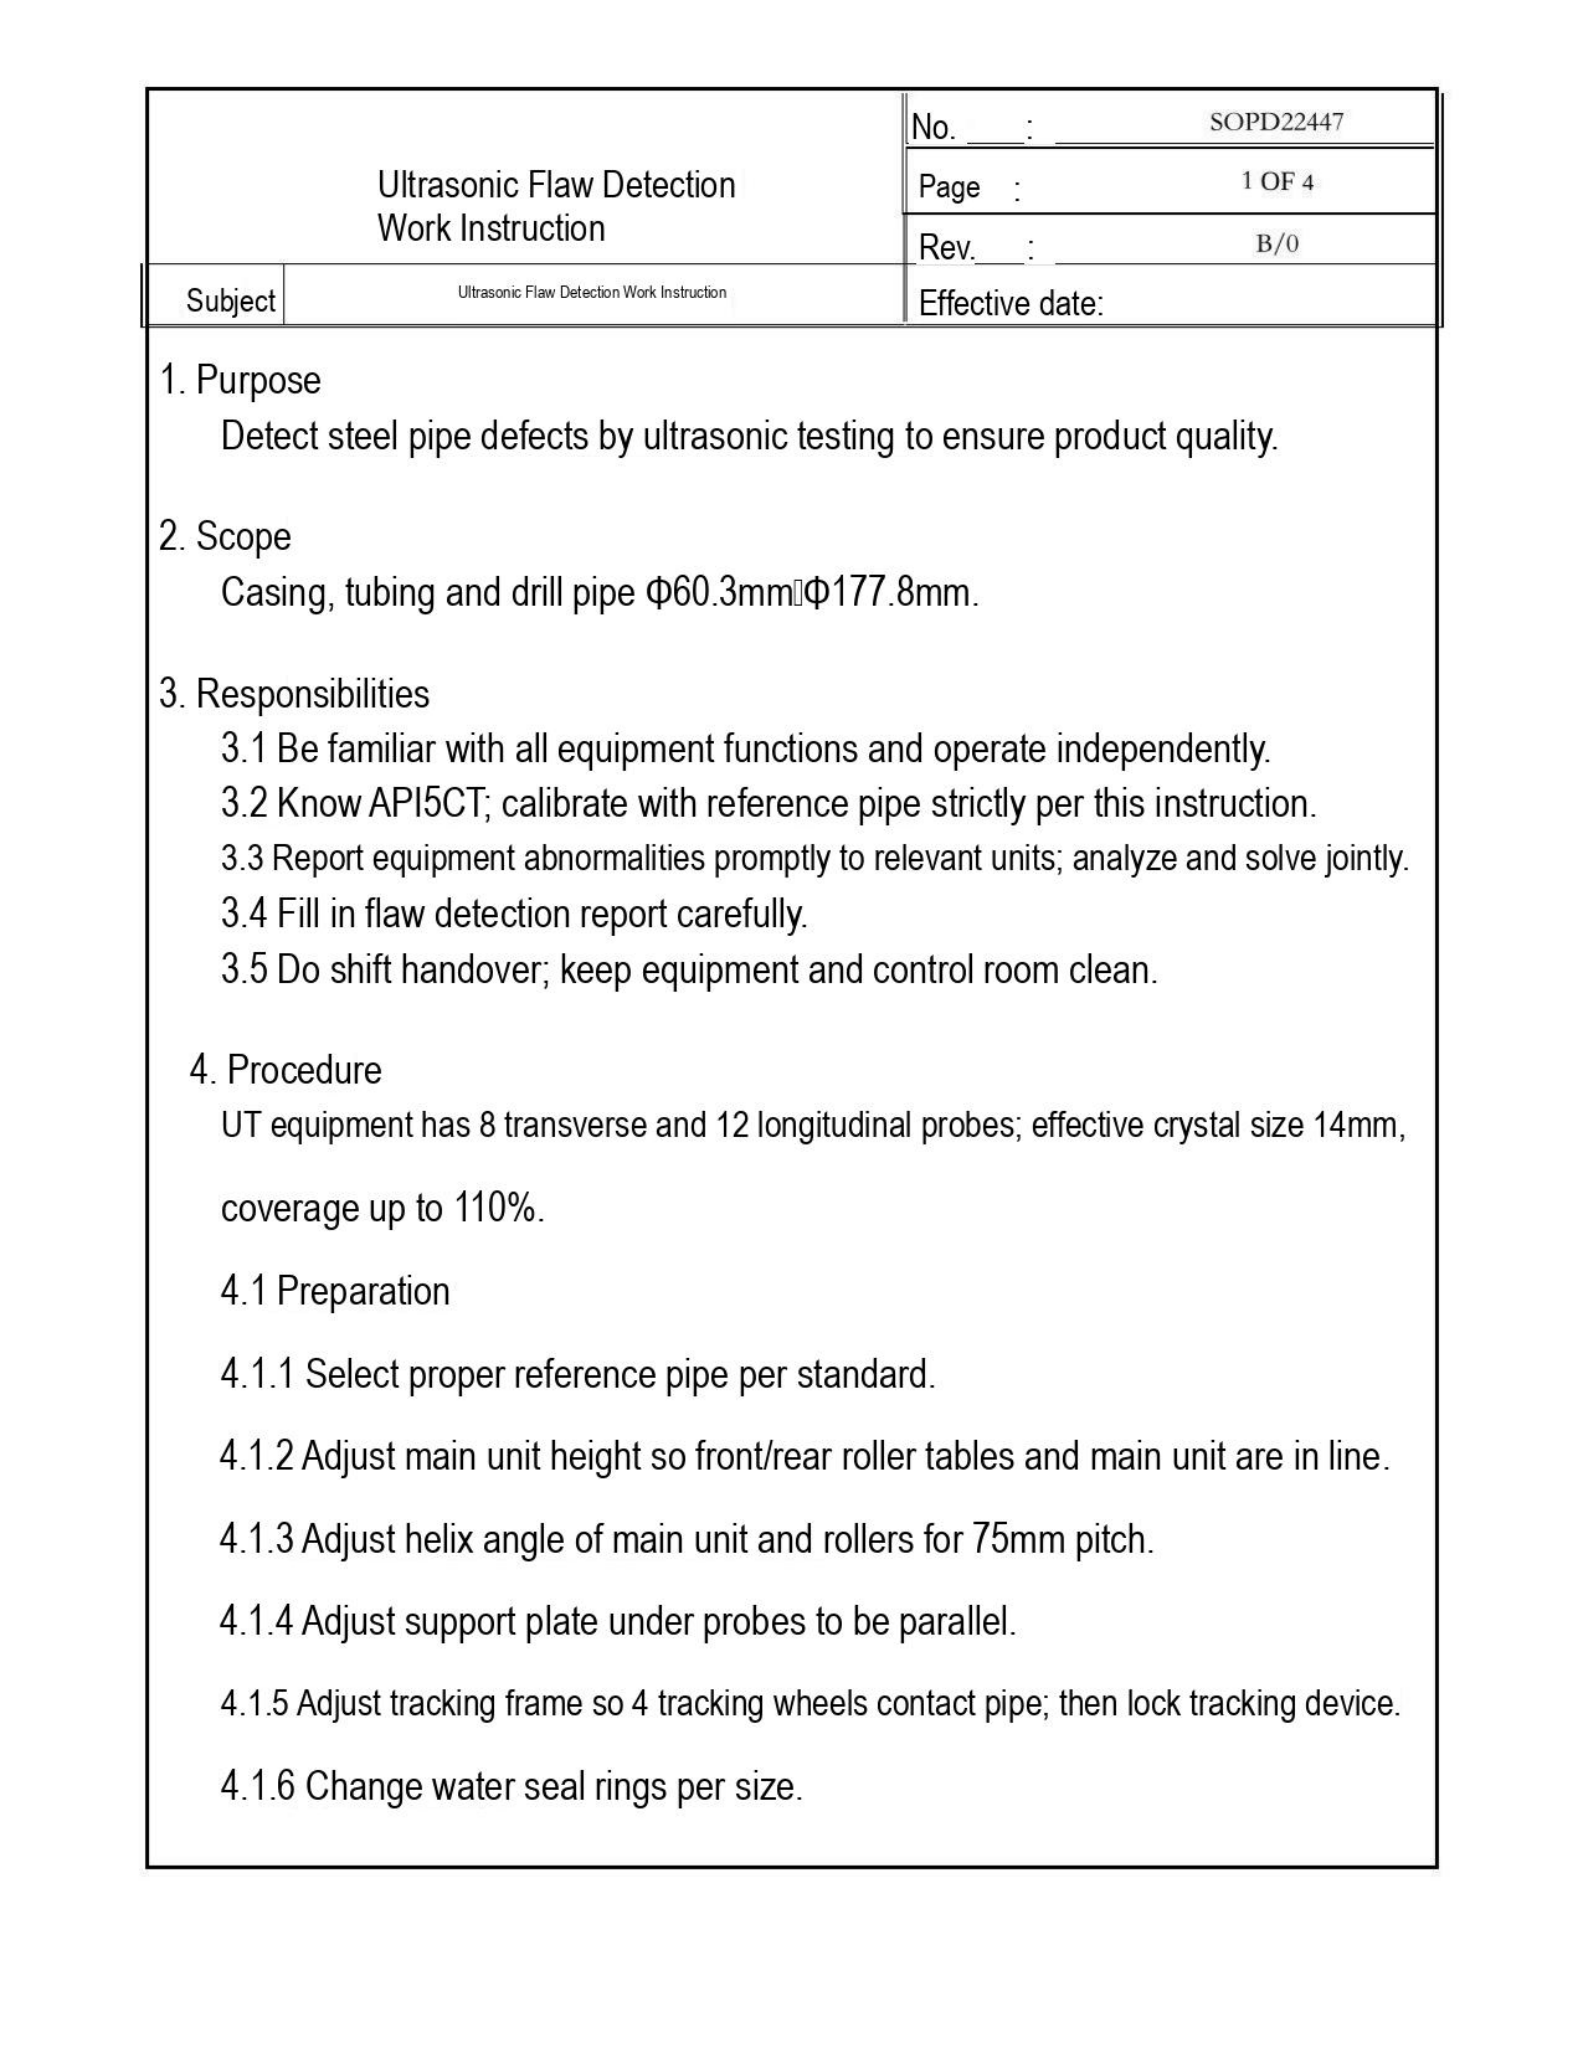| Ultrasonic Flaw Detection Work Instruction | | No. : SOPD22447 |
|---|---|---|
| | | Page : 1 OF 4 |
| | | Rev. : B/0 |
| Subject | Ultrasonic Flaw Detection Work Instruction | Effective date: |

1. Purpose

Detect steel pipe defects by ultrasonic testing to ensure product quality.

2. Scope

Casing, tubing and drill pipe Φ60.3mmΦ177.8mm.

3. Responsibilities

3.1 Be familiar with all equipment functions and operate independently.

3.2 Know API5CT; calibrate with reference pipe strictly per this instruction.

3.3 Report equipment abnormalities promptly to relevant units; analyze and solve jointly.

3.4 Fill in flaw detection report carefully.

3.5 Do shift handover; keep equipment and control room clean.

4. Procedure

UT equipment has 8 transverse and 12 longitudinal probes; effective crystal size 14mm, coverage up to 110%.

4.1 Preparation

4.1.1 Select proper reference pipe per standard.

4.1.2 Adjust main unit height so front/rear roller tables and main unit are in line.

4.1.3 Adjust helix angle of main unit and rollers for 75mm pitch.

4.1.4 Adjust support plate under probes to be parallel.

4.1.5 Adjust tracking frame so 4 tracking wheels contact pipe; then lock tracking device.

4.1.6 Change water seal rings per size.
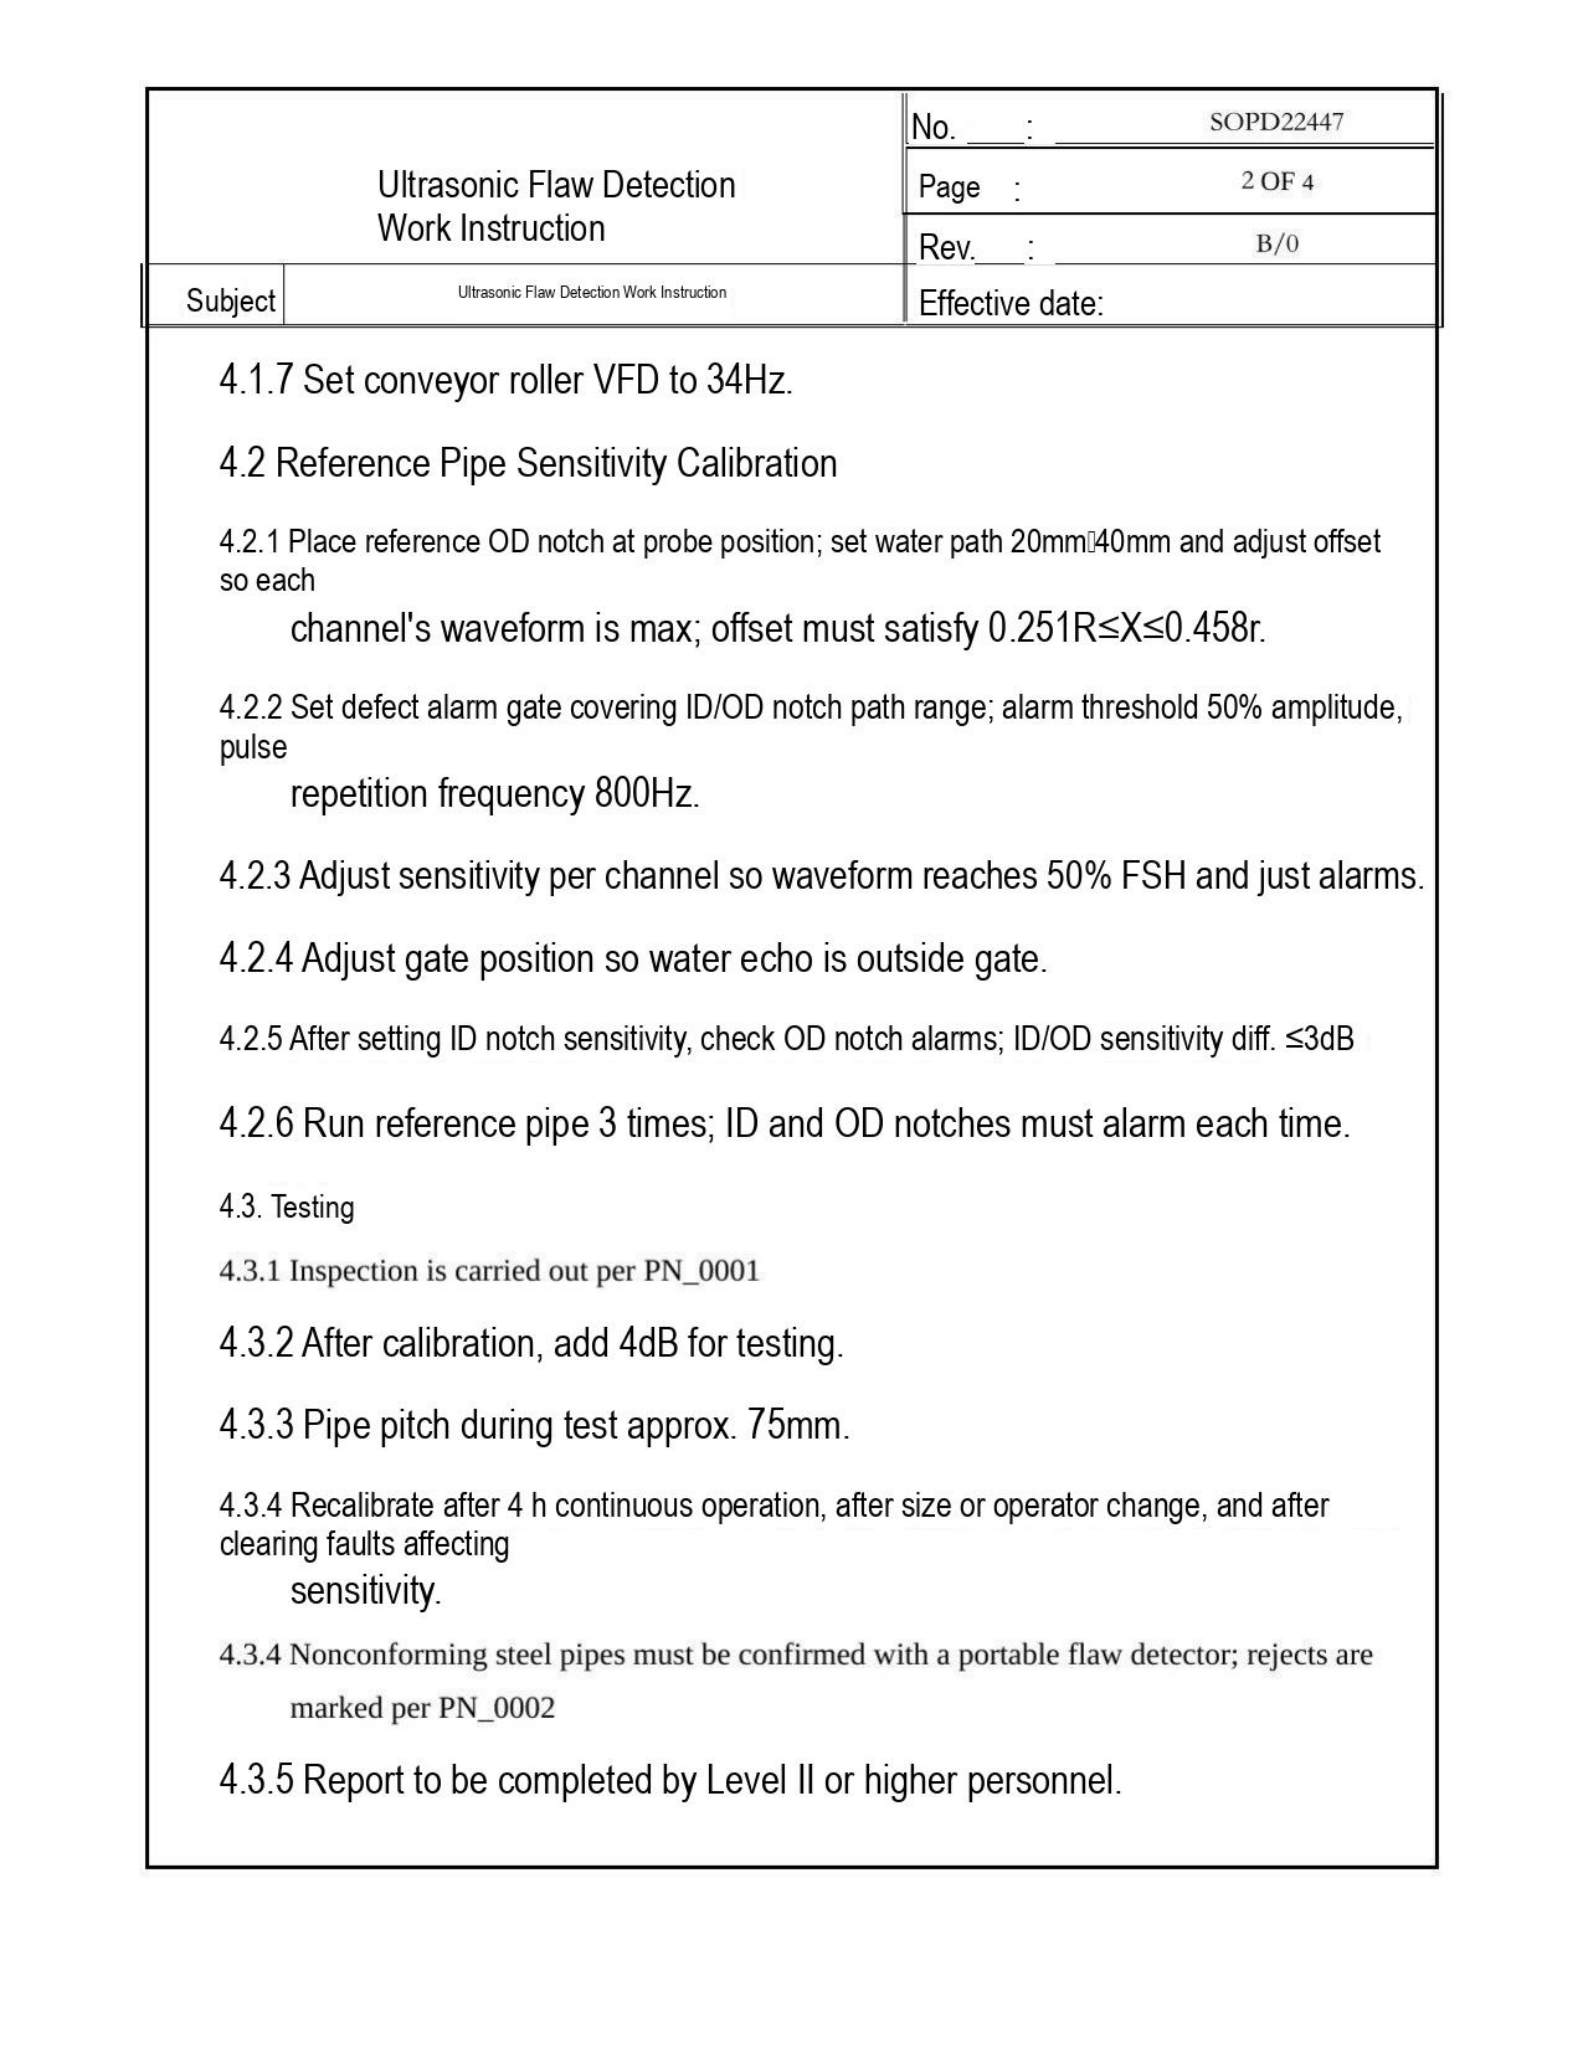| Ultrasonic Flaw Detection Work Instruction | No. : SOPD22447 |
|---|---|
| | Page : 2 OF 4 |
| | Rev. : B/0 |
| Subject: Ultrasonic Flaw Detection Work Instruction | Effective date: |

4.1.7 Set conveyor roller VFD to 34Hz.

4.2 Reference Pipe Sensitivity Calibration

4.2.1 Place reference OD notch at probe position; set water path 20mm□40mm and adjust offset so each channel's waveform is max; offset must satisfy 0.251R≤X≤0.458r.

4.2.2 Set defect alarm gate covering ID/OD notch path range; alarm threshold 50% amplitude, pulse repetition frequency 800Hz.

4.2.3 Adjust sensitivity per channel so waveform reaches 50% FSH and just alarms.

4.2.4 Adjust gate position so water echo is outside gate.

4.2.5 After setting ID notch sensitivity, check OD notch alarms; ID/OD sensitivity diff. ≤3dB

4.2.6 Run reference pipe 3 times; ID and OD notches must alarm each time.

4.3. Testing

4.3.1 Inspection is carried out per PN_0001

4.3.2 After calibration, add 4dB for testing.

4.3.3 Pipe pitch during test approx. 75mm.

4.3.4 Recalibrate after 4 h continuous operation, after size or operator change, and after clearing faults affecting sensitivity.

4.3.4 Nonconforming steel pipes must be confirmed with a portable flaw detector; rejects are marked per PN_0002

4.3.5 Report to be completed by Level II or higher personnel.
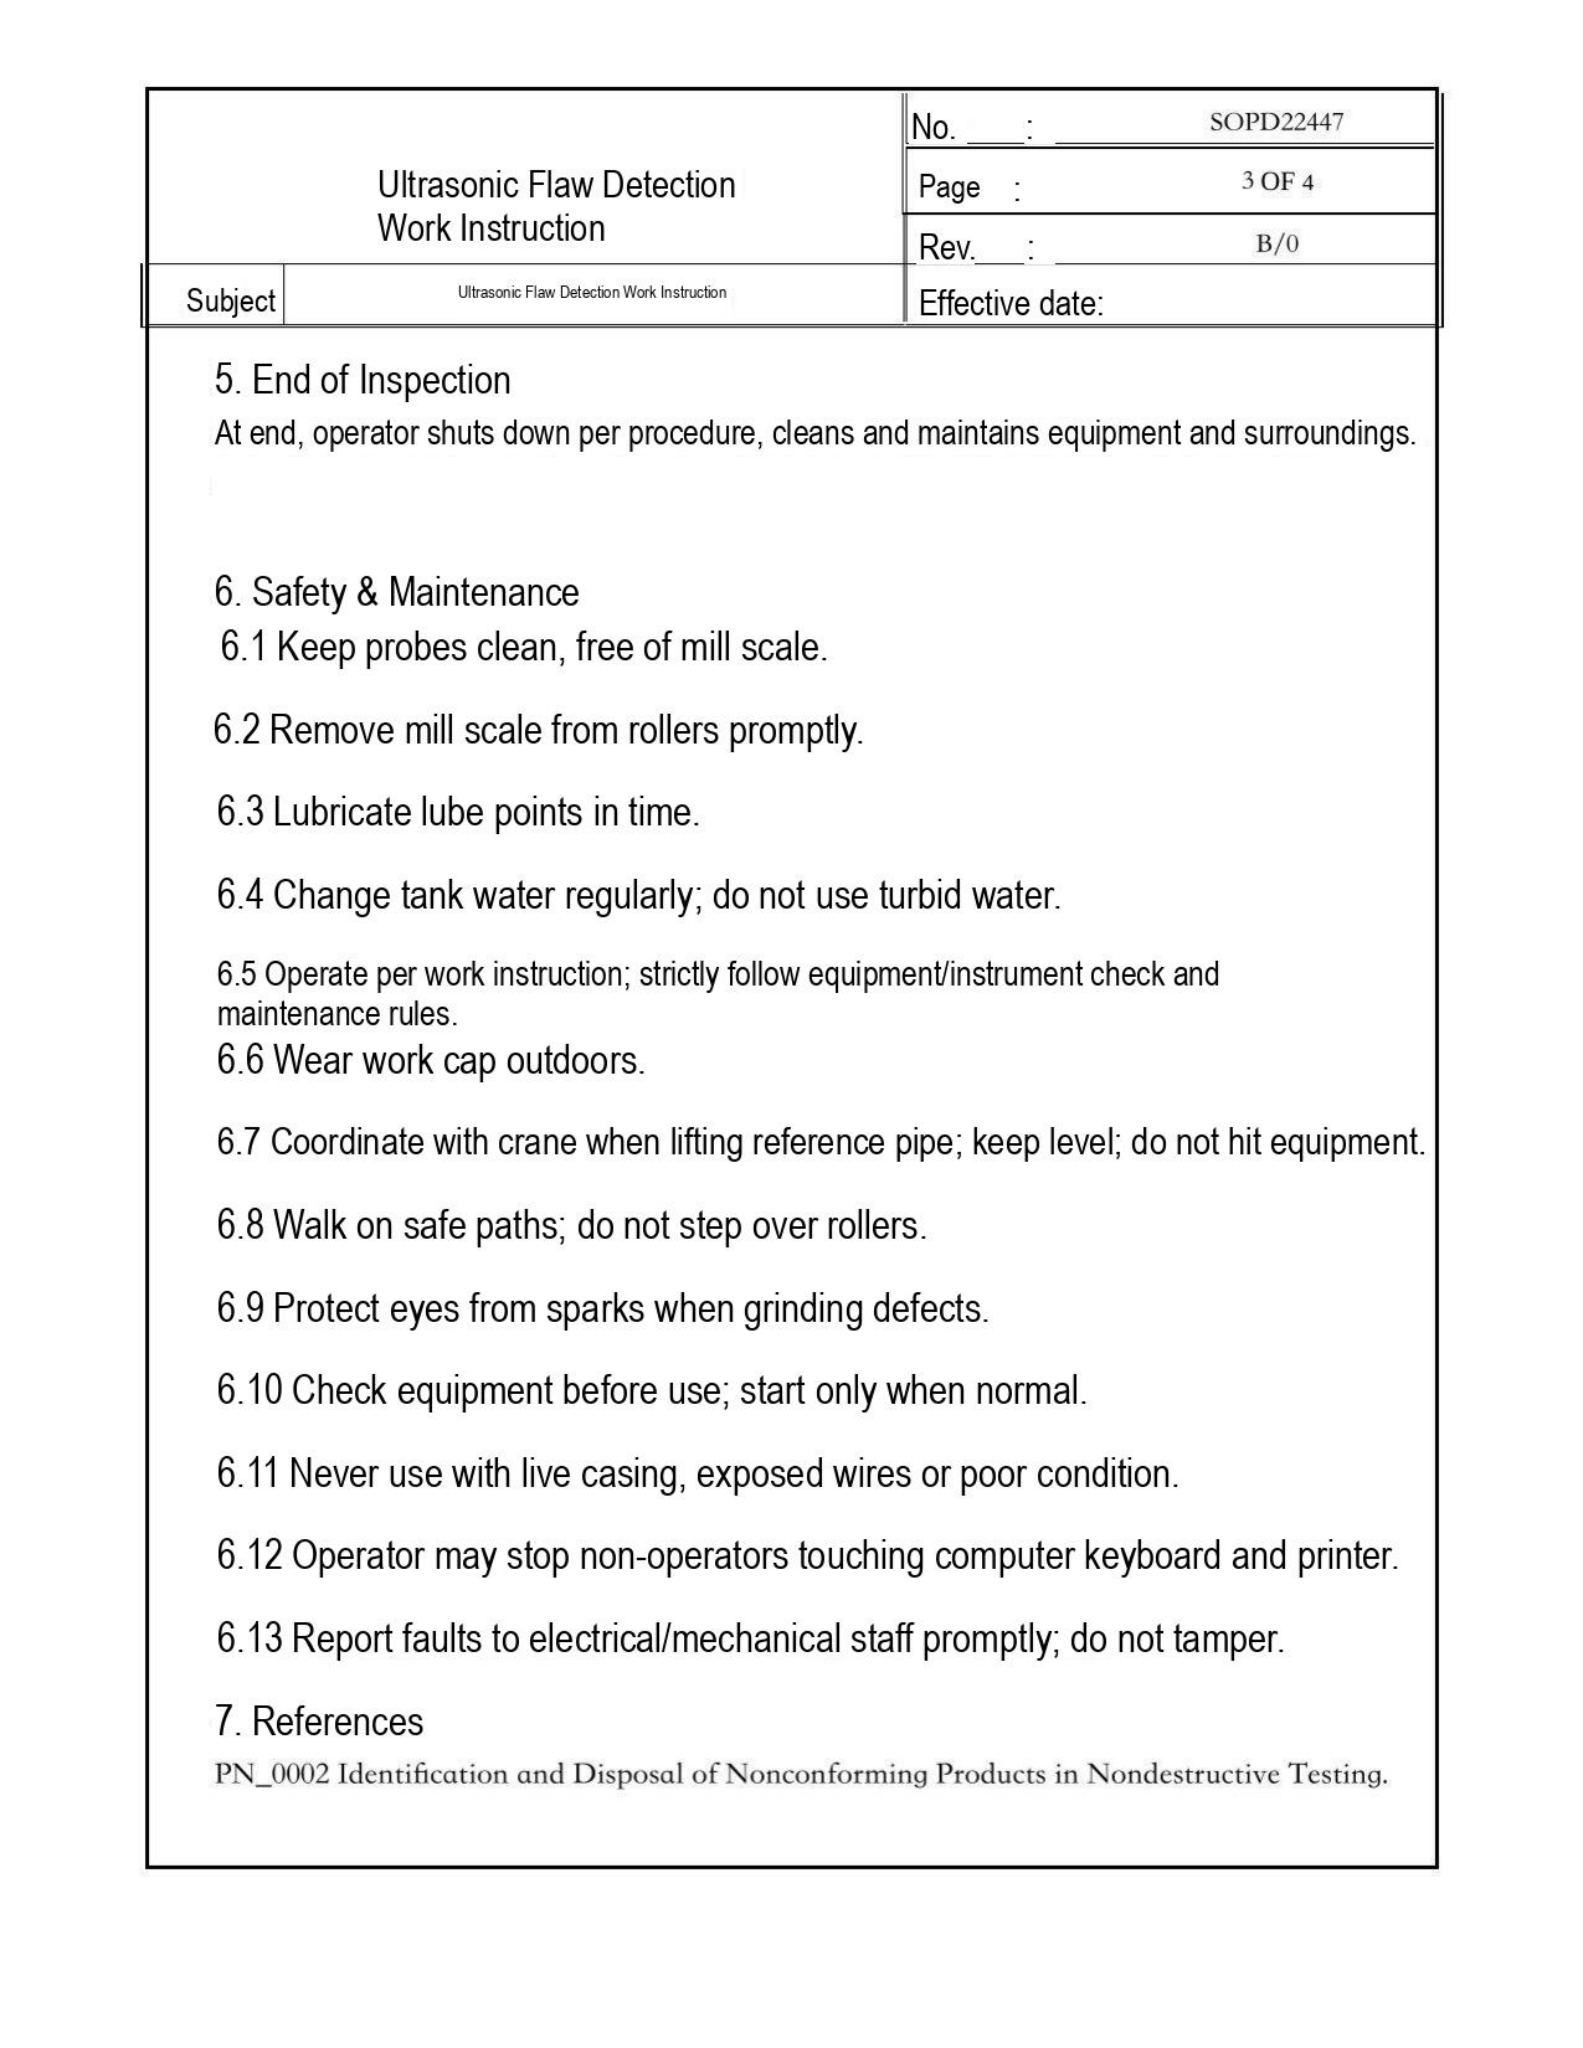| Ultrasonic Flaw Detection Work Instruction | | No. : | SOPD22447 |
|---|---|---|---|
| | | Page : | 3 OF 4 |
| | | Rev. : | B/0 |
| Subject | Ultrasonic Flaw Detection Work Instruction | Effective date: | |

5. End of Inspection
At end, operator shuts down per procedure, cleans and maintains equipment and surroundings.

6. Safety & Maintenance
6.1 Keep probes clean, free of mill scale.

6.2 Remove mill scale from rollers promptly.

6.3 Lubricate lube points in time.

6.4 Change tank water regularly; do not use turbid water.

6.5 Operate per work instruction; strictly follow equipment/instrument check and maintenance rules.
6.6 Wear work cap outdoors.

6.7 Coordinate with crane when lifting reference pipe; keep level; do not hit equipment.

6.8 Walk on safe paths; do not step over rollers.

6.9 Protect eyes from sparks when grinding defects.

6.10 Check equipment before use; start only when normal.

6.11 Never use with live casing, exposed wires or poor condition.

6.12 Operator may stop non-operators touching computer keyboard and printer.

6.13 Report faults to electrical/mechanical staff promptly; do not tamper.

7. References
PN_0002 Identification and Disposal of Nonconforming Products in Nondestructive Testing.
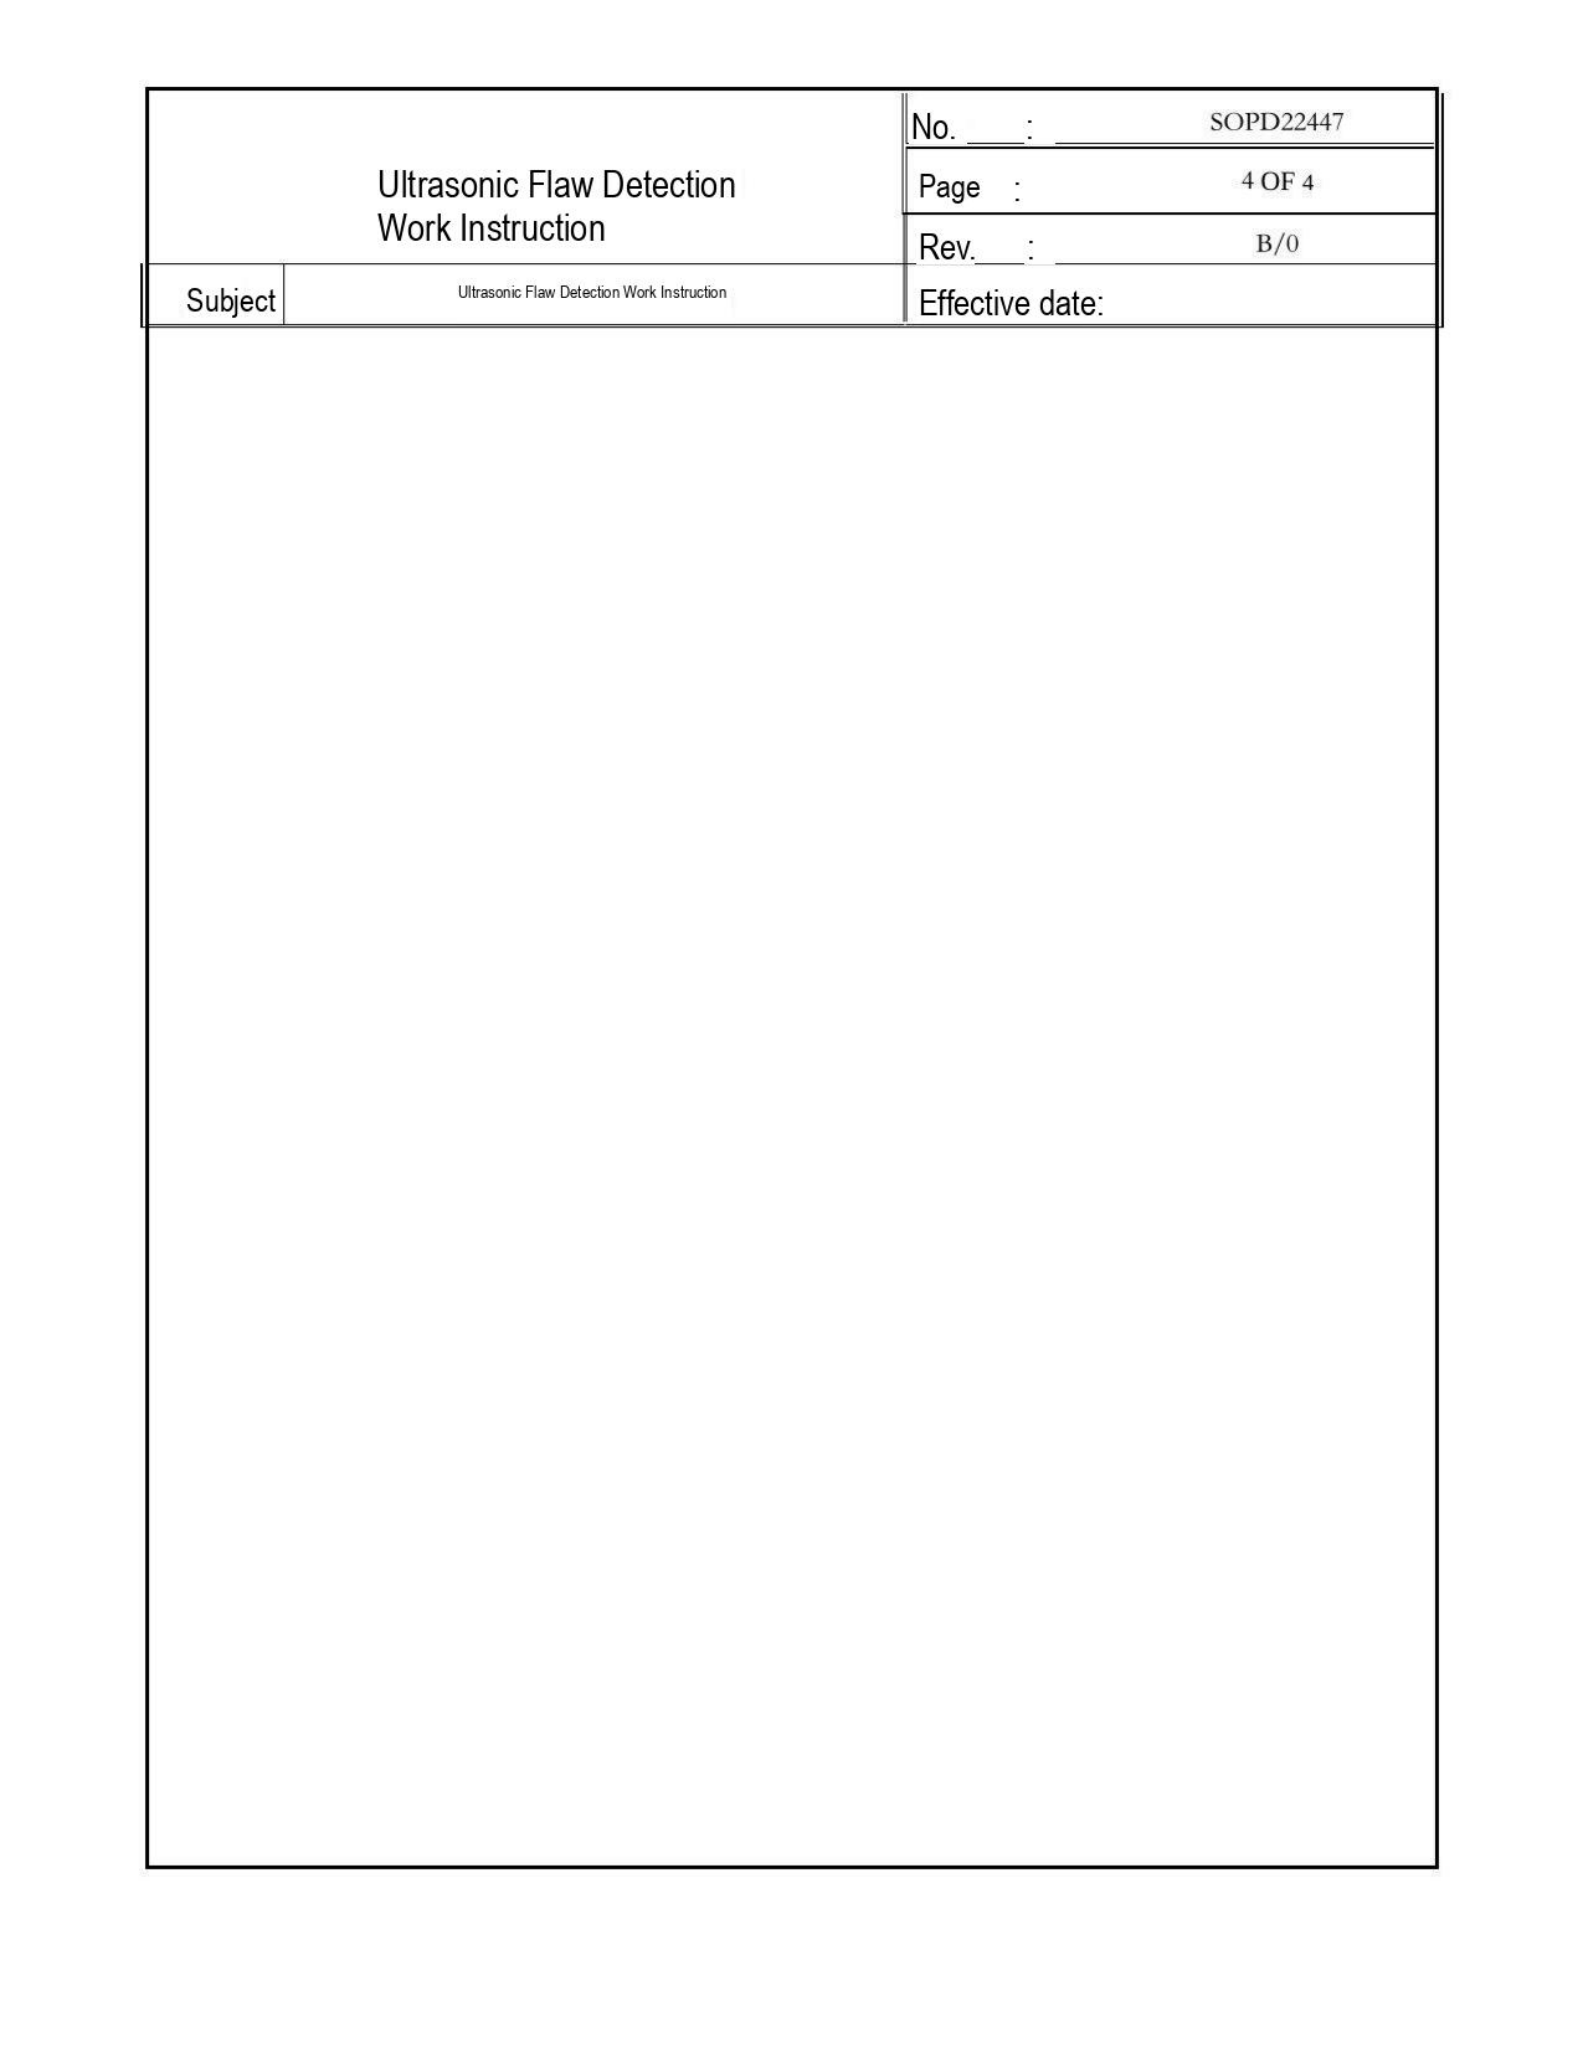| Ultrasonic Flaw Detection Work Instruction | | No. : | SOPD22447 |
|---|---|---|---|
| | | Page : | 4 OF 4 |
| | | Rev. : | B/0 |
| Subject | Ultrasonic Flaw Detection Work Instruction | Effective date: | |